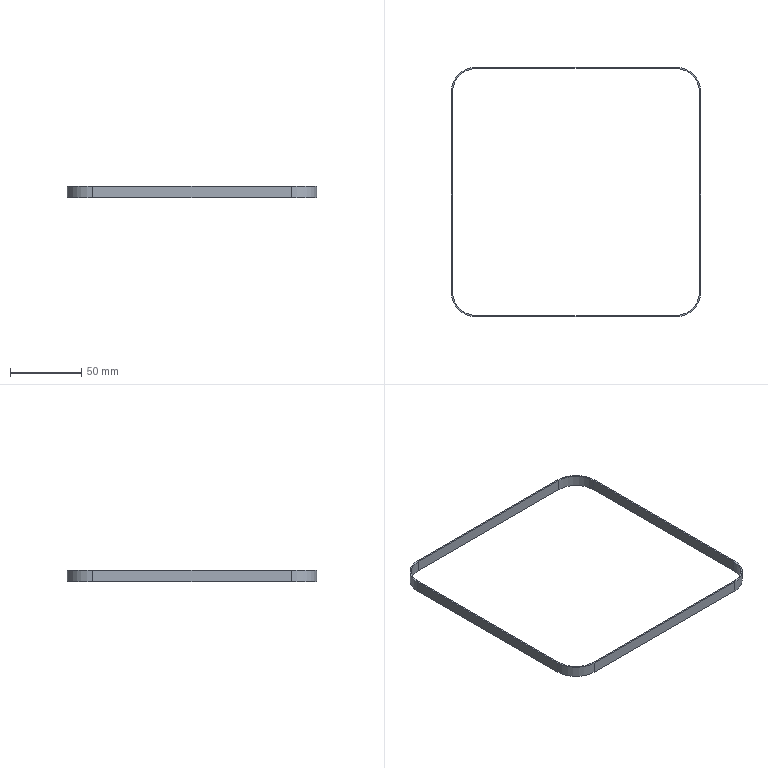Part | NX | features BREP 1 | 1 solid | 18 faces | box 176 x 176 x 7.9 mm | volume 5293 mm3 | plane 10 | cylinder 8 | commonest cylinder face diameters 34 x4 36 x4
STEP:
#1=CARTESIAN_POINT('',(105.422,99.098,7.9));
#2=VERTEX_POINT('',#1);
#3=CARTESIAN_POINT('',(87.422,117.098,7.9));
#4=VERTEX_POINT('',#3);
#5=CARTESIAN_POINT('',(87.422,99.098,7.9));
#6=DIRECTION('',(0.,0.,1.));
#7=DIRECTION('',(1.,0.,0.));
#8=AXIS2_PLACEMENT_3D('',#5,#6,#7);
#9=CIRCLE('',#8,18.);
#10=EDGE_CURVE('',#2,#4,#9,.T.);
#11=ORIENTED_EDGE('',*,*,#10,.T.);
#12=CARTESIAN_POINT('',(-52.578,117.098,7.9));
#13=VERTEX_POINT('',#12);
#14=CARTESIAN_POINT('',(87.422,117.098,7.9));
#15=DIRECTION('',(-1.,0.,0.));
#16=VECTOR('',#15,1000.);
#17=LINE('',#14,#16);
#18=EDGE_CURVE('',#4,#13,#17,.T.);
#19=ORIENTED_EDGE('',*,*,#18,.T.);
#20=CARTESIAN_POINT('',(-70.578,99.098,7.9));
#21=VERTEX_POINT('',#20);
#22=CARTESIAN_POINT('',(-52.578,99.098,7.9));
#23=DIRECTION('',(0.,0.,1.));
#24=DIRECTION('',(1.,0.,0.));
#25=AXIS2_PLACEMENT_3D('',#22,#23,#24);
#26=CIRCLE('',#25,18.);
#27=EDGE_CURVE('',#13,#21,#26,.T.);
#28=ORIENTED_EDGE('',*,*,#27,.T.);
#29=CARTESIAN_POINT('',(-70.578,-40.902,7.9));
#30=VERTEX_POINT('',#29);
#31=CARTESIAN_POINT('',(-70.578,99.098,7.9));
#32=DIRECTION('',(0.,-1.,0.));
#33=VECTOR('',#32,1000.);
#34=LINE('',#31,#33);
#35=EDGE_CURVE('',#21,#30,#34,.T.);
#36=ORIENTED_EDGE('',*,*,#35,.T.);
#37=CARTESIAN_POINT('',(-52.578,-58.902,7.9));
#38=VERTEX_POINT('',#37);
#39=CARTESIAN_POINT('',(-52.578,-40.902,7.9));
#40=DIRECTION('',(0.,0.,1.));
#41=DIRECTION('',(1.,0.,0.));
#42=AXIS2_PLACEMENT_3D('',#39,#40,#41);
#43=CIRCLE('',#42,18.);
#44=EDGE_CURVE('',#30,#38,#43,.T.);
#45=ORIENTED_EDGE('',*,*,#44,.T.);
#46=CARTESIAN_POINT('',(87.422,-58.902,7.9));
#47=VERTEX_POINT('',#46);
#48=CARTESIAN_POINT('',(-52.578,-58.902,7.9));
#49=DIRECTION('',(1.,0.,0.));
#50=VECTOR('',#49,1000.);
#51=LINE('',#48,#50);
#52=EDGE_CURVE('',#38,#47,#51,.T.);
#53=ORIENTED_EDGE('',*,*,#52,.T.);
#54=CARTESIAN_POINT('',(105.422,-40.902,7.9));
#55=VERTEX_POINT('',#54);
#56=CARTESIAN_POINT('',(87.422,-40.902,7.9));
#57=DIRECTION('',(0.,0.,1.));
#58=DIRECTION('',(1.,0.,0.));
#59=AXIS2_PLACEMENT_3D('',#56,#57,#58);
#60=CIRCLE('',#59,18.);
#61=EDGE_CURVE('',#47,#55,#60,.T.);
#62=ORIENTED_EDGE('',*,*,#61,.T.);
#63=CARTESIAN_POINT('',(105.422,-40.902,7.9));
#64=DIRECTION('',(0.,1.,0.));
#65=VECTOR('',#64,1000.);
#66=LINE('',#63,#65);
#67=EDGE_CURVE('',#55,#2,#66,.T.);
#68=ORIENTED_EDGE('',*,*,#67,.T.);
#69=EDGE_LOOP('',(#11,#19,#28,#36,#45,#53,#62,#68));
#70=FACE_BOUND('',#69,.T.);
#71=CARTESIAN_POINT('',(104.422,-40.902,7.9));
#72=VERTEX_POINT('',#71);
#73=CARTESIAN_POINT('',(104.422,99.098,7.9));
#74=VERTEX_POINT('',#73);
#75=CARTESIAN_POINT('',(104.422,-40.902,7.9));
#76=DIRECTION('',(0.,1.,0.));
#77=VECTOR('',#76,1000.);
#78=LINE('',#75,#77);
#79=EDGE_CURVE('',#72,#74,#78,.T.);
#80=ORIENTED_EDGE('',*,*,#79,.F.);
#81=CARTESIAN_POINT('',(87.422,-57.902,7.9));
#82=VERTEX_POINT('',#81);
#83=CARTESIAN_POINT('',(87.422,-40.902,7.9));
#84=DIRECTION('',(0.,0.,1.));
#85=DIRECTION('',(1.,0.,0.));
#86=AXIS2_PLACEMENT_3D('',#83,#84,#85);
#87=CIRCLE('',#86,17.);
#88=EDGE_CURVE('',#82,#72,#87,.T.);
#89=ORIENTED_EDGE('',*,*,#88,.F.);
#90=CARTESIAN_POINT('',(-52.578,-57.902,7.9));
#91=VERTEX_POINT('',#90);
#92=CARTESIAN_POINT('',(-52.578,-57.902,7.9));
#93=DIRECTION('',(1.,0.,0.));
#94=VECTOR('',#93,1000.);
#95=LINE('',#92,#94);
#96=EDGE_CURVE('',#91,#82,#95,.T.);
#97=ORIENTED_EDGE('',*,*,#96,.F.);
#98=CARTESIAN_POINT('',(-69.578,-40.902,7.9));
#99=VERTEX_POINT('',#98);
#100=CARTESIAN_POINT('',(-52.578,-40.902,7.9));
#101=DIRECTION('',(0.,0.,1.));
#102=DIRECTION('',(1.,0.,0.));
#103=AXIS2_PLACEMENT_3D('',#100,#101,#102);
#104=CIRCLE('',#103,17.);
#105=EDGE_CURVE('',#99,#91,#104,.T.);
#106=ORIENTED_EDGE('',*,*,#105,.F.);
#107=CARTESIAN_POINT('',(-69.578,99.098,7.9));
#108=VERTEX_POINT('',#107);
#109=CARTESIAN_POINT('',(-69.578,99.098,7.9));
#110=DIRECTION('',(0.,-1.,0.));
#111=VECTOR('',#110,1000.);
#112=LINE('',#109,#111);
#113=EDGE_CURVE('',#108,#99,#112,.T.);
#114=ORIENTED_EDGE('',*,*,#113,.F.);
#115=CARTESIAN_POINT('',(-52.578,116.098,7.9));
#116=VERTEX_POINT('',#115);
#117=CARTESIAN_POINT('',(-52.578,99.098,7.9));
#118=DIRECTION('',(0.,0.,1.));
#119=DIRECTION('',(1.,0.,0.));
#120=AXIS2_PLACEMENT_3D('',#117,#118,#119);
#121=CIRCLE('',#120,17.);
#122=EDGE_CURVE('',#116,#108,#121,.T.);
#123=ORIENTED_EDGE('',*,*,#122,.F.);
#124=CARTESIAN_POINT('',(87.422,116.098,7.9));
#125=VERTEX_POINT('',#124);
#126=CARTESIAN_POINT('',(87.422,116.098,7.9));
#127=DIRECTION('',(-1.,0.,0.));
#128=VECTOR('',#127,1000.);
#129=LINE('',#126,#128);
#130=EDGE_CURVE('',#125,#116,#129,.T.);
#131=ORIENTED_EDGE('',*,*,#130,.F.);
#132=CARTESIAN_POINT('',(87.422,99.098,7.9));
#133=DIRECTION('',(0.,0.,1.));
#134=DIRECTION('',(1.,0.,0.));
#135=AXIS2_PLACEMENT_3D('',#132,#133,#134);
#136=CIRCLE('',#135,17.);
#137=EDGE_CURVE('',#74,#125,#136,.T.);
#138=ORIENTED_EDGE('',*,*,#137,.F.);
#139=EDGE_LOOP('',(#80,#89,#97,#106,#114,#123,#131,#138));
#140=FACE_BOUND('',#139,.T.);
#141=CARTESIAN_POINT('',(87.422,99.098,7.9));
#142=DIRECTION('',(0.,0.,1.));
#143=DIRECTION('',(-1.,0.,0.));
#144=AXIS2_PLACEMENT_3D('',#141,#142,#143);
#145=PLANE('',#144);
#146=ADVANCED_FACE('',(#70,#140),#145,.T.);
#147=CARTESIAN_POINT('',(105.422,99.098,0.));
#148=VERTEX_POINT('',#147);
#149=CARTESIAN_POINT('',(87.422,117.098,0.));
#150=VERTEX_POINT('',#149);
#151=CARTESIAN_POINT('',(87.422,99.098,0.));
#152=DIRECTION('',(0.,0.,1.));
#153=DIRECTION('',(1.,0.,0.));
#154=AXIS2_PLACEMENT_3D('',#151,#152,#153);
#155=CIRCLE('',#154,18.);
#156=EDGE_CURVE('',#148,#150,#155,.T.);
#157=ORIENTED_EDGE('',*,*,#156,.F.);
#158=CARTESIAN_POINT('',(105.422,-40.902,0.));
#159=VERTEX_POINT('',#158);
#160=CARTESIAN_POINT('',(105.422,-40.902,0.));
#161=DIRECTION('',(0.,1.,0.));
#162=VECTOR('',#161,1000.);
#163=LINE('',#160,#162);
#164=EDGE_CURVE('',#159,#148,#163,.T.);
#165=ORIENTED_EDGE('',*,*,#164,.F.);
#166=CARTESIAN_POINT('',(87.422,-58.902,0.));
#167=VERTEX_POINT('',#166);
#168=CARTESIAN_POINT('',(87.422,-40.902,0.));
#169=DIRECTION('',(0.,0.,1.));
#170=DIRECTION('',(1.,0.,0.));
#171=AXIS2_PLACEMENT_3D('',#168,#169,#170);
#172=CIRCLE('',#171,18.);
#173=EDGE_CURVE('',#167,#159,#172,.T.);
#174=ORIENTED_EDGE('',*,*,#173,.F.);
#175=CARTESIAN_POINT('',(-52.578,-58.902,0.));
#176=VERTEX_POINT('',#175);
#177=CARTESIAN_POINT('',(-52.578,-58.902,0.));
#178=DIRECTION('',(1.,0.,0.));
#179=VECTOR('',#178,1000.);
#180=LINE('',#177,#179);
#181=EDGE_CURVE('',#176,#167,#180,.T.);
#182=ORIENTED_EDGE('',*,*,#181,.F.);
#183=CARTESIAN_POINT('',(-70.578,-40.902,0.));
#184=VERTEX_POINT('',#183);
#185=CARTESIAN_POINT('',(-52.578,-40.902,0.));
#186=DIRECTION('',(0.,0.,1.));
#187=DIRECTION('',(1.,0.,0.));
#188=AXIS2_PLACEMENT_3D('',#185,#186,#187);
#189=CIRCLE('',#188,18.);
#190=EDGE_CURVE('',#184,#176,#189,.T.);
#191=ORIENTED_EDGE('',*,*,#190,.F.);
#192=CARTESIAN_POINT('',(-70.578,99.098,0.));
#193=VERTEX_POINT('',#192);
#194=CARTESIAN_POINT('',(-70.578,99.098,0.));
#195=DIRECTION('',(0.,-1.,0.));
#196=VECTOR('',#195,1000.);
#197=LINE('',#194,#196);
#198=EDGE_CURVE('',#193,#184,#197,.T.);
#199=ORIENTED_EDGE('',*,*,#198,.F.);
#200=CARTESIAN_POINT('',(-52.578,117.098,0.));
#201=VERTEX_POINT('',#200);
#202=CARTESIAN_POINT('',(-52.578,99.098,0.));
#203=DIRECTION('',(0.,0.,1.));
#204=DIRECTION('',(1.,0.,0.));
#205=AXIS2_PLACEMENT_3D('',#202,#203,#204);
#206=CIRCLE('',#205,18.);
#207=EDGE_CURVE('',#201,#193,#206,.T.);
#208=ORIENTED_EDGE('',*,*,#207,.F.);
#209=CARTESIAN_POINT('',(87.422,117.098,0.));
#210=DIRECTION('',(-1.,0.,0.));
#211=VECTOR('',#210,1000.);
#212=LINE('',#209,#211);
#213=EDGE_CURVE('',#150,#201,#212,.T.);
#214=ORIENTED_EDGE('',*,*,#213,.F.);
#215=EDGE_LOOP('',(#157,#165,#174,#182,#191,#199,#208,#214));
#216=FACE_BOUND('',#215,.T.);
#217=CARTESIAN_POINT('',(87.422,-57.902,0.));
#218=VERTEX_POINT('',#217);
#219=CARTESIAN_POINT('',(104.422,-40.902,0.));
#220=VERTEX_POINT('',#219);
#221=CARTESIAN_POINT('',(87.422,-40.902,0.));
#222=DIRECTION('',(0.,0.,1.));
#223=DIRECTION('',(1.,0.,0.));
#224=AXIS2_PLACEMENT_3D('',#221,#222,#223);
#225=CIRCLE('',#224,17.);
#226=EDGE_CURVE('',#218,#220,#225,.T.);
#227=ORIENTED_EDGE('',*,*,#226,.T.);
#228=CARTESIAN_POINT('',(104.422,99.098,0.));
#229=VERTEX_POINT('',#228);
#230=CARTESIAN_POINT('',(104.422,-40.902,0.));
#231=DIRECTION('',(0.,1.,0.));
#232=VECTOR('',#231,1000.);
#233=LINE('',#230,#232);
#234=EDGE_CURVE('',#220,#229,#233,.T.);
#235=ORIENTED_EDGE('',*,*,#234,.T.);
#236=CARTESIAN_POINT('',(87.422,116.098,0.));
#237=VERTEX_POINT('',#236);
#238=CARTESIAN_POINT('',(87.422,99.098,0.));
#239=DIRECTION('',(0.,0.,1.));
#240=DIRECTION('',(1.,0.,0.));
#241=AXIS2_PLACEMENT_3D('',#238,#239,#240);
#242=CIRCLE('',#241,17.);
#243=EDGE_CURVE('',#229,#237,#242,.T.);
#244=ORIENTED_EDGE('',*,*,#243,.T.);
#245=CARTESIAN_POINT('',(-52.578,116.098,0.));
#246=VERTEX_POINT('',#245);
#247=CARTESIAN_POINT('',(87.422,116.098,0.));
#248=DIRECTION('',(-1.,0.,0.));
#249=VECTOR('',#248,1000.);
#250=LINE('',#247,#249);
#251=EDGE_CURVE('',#237,#246,#250,.T.);
#252=ORIENTED_EDGE('',*,*,#251,.T.);
#253=CARTESIAN_POINT('',(-69.578,99.098,0.));
#254=VERTEX_POINT('',#253);
#255=CARTESIAN_POINT('',(-52.578,99.098,0.));
#256=DIRECTION('',(0.,0.,1.));
#257=DIRECTION('',(1.,0.,0.));
#258=AXIS2_PLACEMENT_3D('',#255,#256,#257);
#259=CIRCLE('',#258,17.);
#260=EDGE_CURVE('',#246,#254,#259,.T.);
#261=ORIENTED_EDGE('',*,*,#260,.T.);
#262=CARTESIAN_POINT('',(-69.578,-40.902,0.));
#263=VERTEX_POINT('',#262);
#264=CARTESIAN_POINT('',(-69.578,99.098,0.));
#265=DIRECTION('',(0.,-1.,0.));
#266=VECTOR('',#265,1000.);
#267=LINE('',#264,#266);
#268=EDGE_CURVE('',#254,#263,#267,.T.);
#269=ORIENTED_EDGE('',*,*,#268,.T.);
#270=CARTESIAN_POINT('',(-52.578,-57.902,0.));
#271=VERTEX_POINT('',#270);
#272=CARTESIAN_POINT('',(-52.578,-40.902,0.));
#273=DIRECTION('',(0.,0.,1.));
#274=DIRECTION('',(1.,0.,0.));
#275=AXIS2_PLACEMENT_3D('',#272,#273,#274);
#276=CIRCLE('',#275,17.);
#277=EDGE_CURVE('',#263,#271,#276,.T.);
#278=ORIENTED_EDGE('',*,*,#277,.T.);
#279=CARTESIAN_POINT('',(-52.578,-57.902,0.));
#280=DIRECTION('',(1.,0.,0.));
#281=VECTOR('',#280,1000.);
#282=LINE('',#279,#281);
#283=EDGE_CURVE('',#271,#218,#282,.T.);
#284=ORIENTED_EDGE('',*,*,#283,.T.);
#285=EDGE_LOOP('',(#227,#235,#244,#252,#261,#269,#278,#284));
#286=FACE_BOUND('',#285,.T.);
#287=CARTESIAN_POINT('',(87.422,99.098,0.));
#288=DIRECTION('',(0.,0.,1.));
#289=DIRECTION('',(-1.,0.,0.));
#290=AXIS2_PLACEMENT_3D('',#287,#288,#289);
#291=PLANE('',#290);
#292=ADVANCED_FACE('',(#216,#286),#291,.F.);
#293=ORIENTED_EDGE('',*,*,#156,.T.);
#294=CARTESIAN_POINT('',(87.422,117.098,7.9));
#295=DIRECTION('',(0.,0.,-1.));
#296=VECTOR('',#295,1000.);
#297=LINE('',#294,#296);
#298=EDGE_CURVE('',#4,#150,#297,.T.);
#299=ORIENTED_EDGE('',*,*,#298,.F.);
#300=ORIENTED_EDGE('',*,*,#10,.F.);
#301=CARTESIAN_POINT('',(105.422,99.098,7.9));
#302=DIRECTION('',(0.,0.,-1.));
#303=VECTOR('',#302,1000.);
#304=LINE('',#301,#303);
#305=EDGE_CURVE('',#2,#148,#304,.T.);
#306=ORIENTED_EDGE('',*,*,#305,.T.);
#307=EDGE_LOOP('',(#293,#299,#300,#306));
#308=FACE_BOUND('',#307,.T.);
#309=CARTESIAN_POINT('',(87.422,99.098,7.9));
#310=DIRECTION('',(0.,0.,-1.));
#311=DIRECTION('',(1.,0.,0.));
#312=AXIS2_PLACEMENT_3D('',#309,#310,#311);
#313=CYLINDRICAL_SURFACE('',#312,18.);
#314=ADVANCED_FACE('',(#308),#313,.T.);
#315=ORIENTED_EDGE('',*,*,#213,.T.);
#316=CARTESIAN_POINT('',(-52.578,117.098,7.9));
#317=DIRECTION('',(0.,0.,-1.));
#318=VECTOR('',#317,1000.);
#319=LINE('',#316,#318);
#320=EDGE_CURVE('',#13,#201,#319,.T.);
#321=ORIENTED_EDGE('',*,*,#320,.F.);
#322=ORIENTED_EDGE('',*,*,#18,.F.);
#323=ORIENTED_EDGE('',*,*,#298,.T.);
#324=EDGE_LOOP('',(#315,#321,#322,#323));
#325=FACE_BOUND('',#324,.T.);
#326=CARTESIAN_POINT('',(87.422,117.098,7.9));
#327=DIRECTION('',(0.,-1.,0.));
#328=DIRECTION('',(0.,0.,1.));
#329=AXIS2_PLACEMENT_3D('',#326,#327,#328);
#330=PLANE('',#329);
#331=ADVANCED_FACE('',(#325),#330,.F.);
#332=ORIENTED_EDGE('',*,*,#207,.T.);
#333=CARTESIAN_POINT('',(-70.578,99.098,7.9));
#334=DIRECTION('',(0.,0.,-1.));
#335=VECTOR('',#334,1000.);
#336=LINE('',#333,#335);
#337=EDGE_CURVE('',#21,#193,#336,.T.);
#338=ORIENTED_EDGE('',*,*,#337,.F.);
#339=ORIENTED_EDGE('',*,*,#27,.F.);
#340=ORIENTED_EDGE('',*,*,#320,.T.);
#341=EDGE_LOOP('',(#332,#338,#339,#340));
#342=FACE_BOUND('',#341,.T.);
#343=CARTESIAN_POINT('',(-52.578,99.098,7.9));
#344=DIRECTION('',(0.,0.,-1.));
#345=DIRECTION('',(1.,0.,0.));
#346=AXIS2_PLACEMENT_3D('',#343,#344,#345);
#347=CYLINDRICAL_SURFACE('',#346,18.);
#348=ADVANCED_FACE('',(#342),#347,.T.);
#349=ORIENTED_EDGE('',*,*,#198,.T.);
#350=CARTESIAN_POINT('',(-70.578,-40.902,7.9));
#351=DIRECTION('',(0.,0.,-1.));
#352=VECTOR('',#351,1000.);
#353=LINE('',#350,#352);
#354=EDGE_CURVE('',#30,#184,#353,.T.);
#355=ORIENTED_EDGE('',*,*,#354,.F.);
#356=ORIENTED_EDGE('',*,*,#35,.F.);
#357=ORIENTED_EDGE('',*,*,#337,.T.);
#358=EDGE_LOOP('',(#349,#355,#356,#357));
#359=FACE_BOUND('',#358,.T.);
#360=CARTESIAN_POINT('',(-70.578,99.098,7.9));
#361=DIRECTION('',(1.,0.,0.));
#362=DIRECTION('',(0.,-1.,0.));
#363=AXIS2_PLACEMENT_3D('',#360,#361,#362);
#364=PLANE('',#363);
#365=ADVANCED_FACE('',(#359),#364,.F.);
#366=ORIENTED_EDGE('',*,*,#190,.T.);
#367=CARTESIAN_POINT('',(-52.578,-58.902,7.9));
#368=DIRECTION('',(0.,0.,-1.));
#369=VECTOR('',#368,1000.);
#370=LINE('',#367,#369);
#371=EDGE_CURVE('',#38,#176,#370,.T.);
#372=ORIENTED_EDGE('',*,*,#371,.F.);
#373=ORIENTED_EDGE('',*,*,#44,.F.);
#374=ORIENTED_EDGE('',*,*,#354,.T.);
#375=EDGE_LOOP('',(#366,#372,#373,#374));
#376=FACE_BOUND('',#375,.T.);
#377=CARTESIAN_POINT('',(-52.578,-40.902,7.9));
#378=DIRECTION('',(0.,0.,-1.));
#379=DIRECTION('',(1.,0.,0.));
#380=AXIS2_PLACEMENT_3D('',#377,#378,#379);
#381=CYLINDRICAL_SURFACE('',#380,18.);
#382=ADVANCED_FACE('',(#376),#381,.T.);
#383=ORIENTED_EDGE('',*,*,#181,.T.);
#384=CARTESIAN_POINT('',(87.422,-58.902,7.9));
#385=DIRECTION('',(0.,0.,-1.));
#386=VECTOR('',#385,1000.);
#387=LINE('',#384,#386);
#388=EDGE_CURVE('',#47,#167,#387,.T.);
#389=ORIENTED_EDGE('',*,*,#388,.F.);
#390=ORIENTED_EDGE('',*,*,#52,.F.);
#391=ORIENTED_EDGE('',*,*,#371,.T.);
#392=EDGE_LOOP('',(#383,#389,#390,#391));
#393=FACE_BOUND('',#392,.T.);
#394=CARTESIAN_POINT('',(-52.578,-58.902,7.9));
#395=DIRECTION('',(0.,1.,0.));
#396=DIRECTION('',(-1.,0.,0.));
#397=AXIS2_PLACEMENT_3D('',#394,#395,#396);
#398=PLANE('',#397);
#399=ADVANCED_FACE('',(#393),#398,.F.);
#400=ORIENTED_EDGE('',*,*,#173,.T.);
#401=CARTESIAN_POINT('',(105.422,-40.902,7.9));
#402=DIRECTION('',(0.,0.,-1.));
#403=VECTOR('',#402,1000.);
#404=LINE('',#401,#403);
#405=EDGE_CURVE('',#55,#159,#404,.T.);
#406=ORIENTED_EDGE('',*,*,#405,.F.);
#407=ORIENTED_EDGE('',*,*,#61,.F.);
#408=ORIENTED_EDGE('',*,*,#388,.T.);
#409=EDGE_LOOP('',(#400,#406,#407,#408));
#410=FACE_BOUND('',#409,.T.);
#411=CARTESIAN_POINT('',(87.422,-40.902,7.9));
#412=DIRECTION('',(0.,0.,-1.));
#413=DIRECTION('',(1.,0.,0.));
#414=AXIS2_PLACEMENT_3D('',#411,#412,#413);
#415=CYLINDRICAL_SURFACE('',#414,18.);
#416=ADVANCED_FACE('',(#410),#415,.T.);
#417=ORIENTED_EDGE('',*,*,#164,.T.);
#418=ORIENTED_EDGE('',*,*,#305,.F.);
#419=ORIENTED_EDGE('',*,*,#67,.F.);
#420=ORIENTED_EDGE('',*,*,#405,.T.);
#421=EDGE_LOOP('',(#417,#418,#419,#420));
#422=FACE_BOUND('',#421,.T.);
#423=CARTESIAN_POINT('',(105.422,-40.902,7.9));
#424=DIRECTION('',(-1.,0.,0.));
#425=DIRECTION('',(0.,0.,-1.));
#426=AXIS2_PLACEMENT_3D('',#423,#424,#425);
#427=PLANE('',#426);
#428=ADVANCED_FACE('',(#422),#427,.F.);
#429=ORIENTED_EDGE('',*,*,#226,.F.);
#430=CARTESIAN_POINT('',(87.422,-57.902,7.9));
#431=DIRECTION('',(0.,0.,-1.));
#432=VECTOR('',#431,1000.);
#433=LINE('',#430,#432);
#434=EDGE_CURVE('',#82,#218,#433,.T.);
#435=ORIENTED_EDGE('',*,*,#434,.F.);
#436=ORIENTED_EDGE('',*,*,#88,.T.);
#437=CARTESIAN_POINT('',(104.422,-40.902,7.9));
#438=DIRECTION('',(0.,0.,-1.));
#439=VECTOR('',#438,1000.);
#440=LINE('',#437,#439);
#441=EDGE_CURVE('',#72,#220,#440,.T.);
#442=ORIENTED_EDGE('',*,*,#441,.T.);
#443=EDGE_LOOP('',(#429,#435,#436,#442));
#444=FACE_BOUND('',#443,.T.);
#445=CARTESIAN_POINT('',(87.422,-40.902,7.9));
#446=DIRECTION('',(0.,0.,-1.));
#447=DIRECTION('',(1.,0.,0.));
#448=AXIS2_PLACEMENT_3D('',#445,#446,#447);
#449=CYLINDRICAL_SURFACE('',#448,17.);
#450=ADVANCED_FACE('',(#444),#449,.F.);
#451=ORIENTED_EDGE('',*,*,#234,.F.);
#452=ORIENTED_EDGE('',*,*,#441,.F.);
#453=ORIENTED_EDGE('',*,*,#79,.T.);
#454=CARTESIAN_POINT('',(104.422,99.098,7.9));
#455=DIRECTION('',(0.,0.,-1.));
#456=VECTOR('',#455,1000.);
#457=LINE('',#454,#456);
#458=EDGE_CURVE('',#74,#229,#457,.T.);
#459=ORIENTED_EDGE('',*,*,#458,.T.);
#460=EDGE_LOOP('',(#451,#452,#453,#459));
#461=FACE_BOUND('',#460,.T.);
#462=CARTESIAN_POINT('',(104.422,-40.902,7.9));
#463=DIRECTION('',(-1.,0.,0.));
#464=DIRECTION('',(0.,0.,-1.));
#465=AXIS2_PLACEMENT_3D('',#462,#463,#464);
#466=PLANE('',#465);
#467=ADVANCED_FACE('',(#461),#466,.T.);
#468=ORIENTED_EDGE('',*,*,#243,.F.);
#469=ORIENTED_EDGE('',*,*,#458,.F.);
#470=ORIENTED_EDGE('',*,*,#137,.T.);
#471=CARTESIAN_POINT('',(87.422,116.098,7.9));
#472=DIRECTION('',(0.,0.,-1.));
#473=VECTOR('',#472,1000.);
#474=LINE('',#471,#473);
#475=EDGE_CURVE('',#125,#237,#474,.T.);
#476=ORIENTED_EDGE('',*,*,#475,.T.);
#477=EDGE_LOOP('',(#468,#469,#470,#476));
#478=FACE_BOUND('',#477,.T.);
#479=CARTESIAN_POINT('',(87.422,99.098,7.9));
#480=DIRECTION('',(0.,0.,-1.));
#481=DIRECTION('',(1.,0.,0.));
#482=AXIS2_PLACEMENT_3D('',#479,#480,#481);
#483=CYLINDRICAL_SURFACE('',#482,17.);
#484=ADVANCED_FACE('',(#478),#483,.F.);
#485=ORIENTED_EDGE('',*,*,#251,.F.);
#486=ORIENTED_EDGE('',*,*,#475,.F.);
#487=ORIENTED_EDGE('',*,*,#130,.T.);
#488=CARTESIAN_POINT('',(-52.578,116.098,7.9));
#489=DIRECTION('',(0.,0.,-1.));
#490=VECTOR('',#489,1000.);
#491=LINE('',#488,#490);
#492=EDGE_CURVE('',#116,#246,#491,.T.);
#493=ORIENTED_EDGE('',*,*,#492,.T.);
#494=EDGE_LOOP('',(#485,#486,#487,#493));
#495=FACE_BOUND('',#494,.T.);
#496=CARTESIAN_POINT('',(87.422,116.098,7.9));
#497=DIRECTION('',(0.,-1.,0.));
#498=DIRECTION('',(0.,0.,1.));
#499=AXIS2_PLACEMENT_3D('',#496,#497,#498);
#500=PLANE('',#499);
#501=ADVANCED_FACE('',(#495),#500,.T.);
#502=ORIENTED_EDGE('',*,*,#260,.F.);
#503=ORIENTED_EDGE('',*,*,#492,.F.);
#504=ORIENTED_EDGE('',*,*,#122,.T.);
#505=CARTESIAN_POINT('',(-69.578,99.098,7.9));
#506=DIRECTION('',(0.,0.,-1.));
#507=VECTOR('',#506,1000.);
#508=LINE('',#505,#507);
#509=EDGE_CURVE('',#108,#254,#508,.T.);
#510=ORIENTED_EDGE('',*,*,#509,.T.);
#511=EDGE_LOOP('',(#502,#503,#504,#510));
#512=FACE_BOUND('',#511,.T.);
#513=CARTESIAN_POINT('',(-52.578,99.098,7.9));
#514=DIRECTION('',(0.,0.,-1.));
#515=DIRECTION('',(1.,0.,0.));
#516=AXIS2_PLACEMENT_3D('',#513,#514,#515);
#517=CYLINDRICAL_SURFACE('',#516,17.);
#518=ADVANCED_FACE('',(#512),#517,.F.);
#519=ORIENTED_EDGE('',*,*,#268,.F.);
#520=ORIENTED_EDGE('',*,*,#509,.F.);
#521=ORIENTED_EDGE('',*,*,#113,.T.);
#522=CARTESIAN_POINT('',(-69.578,-40.902,7.9));
#523=DIRECTION('',(0.,0.,-1.));
#524=VECTOR('',#523,1000.);
#525=LINE('',#522,#524);
#526=EDGE_CURVE('',#99,#263,#525,.T.);
#527=ORIENTED_EDGE('',*,*,#526,.T.);
#528=EDGE_LOOP('',(#519,#520,#521,#527));
#529=FACE_BOUND('',#528,.T.);
#530=CARTESIAN_POINT('',(-69.578,99.098,7.9));
#531=DIRECTION('',(1.,0.,0.));
#532=DIRECTION('',(0.,-1.,0.));
#533=AXIS2_PLACEMENT_3D('',#530,#531,#532);
#534=PLANE('',#533);
#535=ADVANCED_FACE('',(#529),#534,.T.);
#536=ORIENTED_EDGE('',*,*,#277,.F.);
#537=ORIENTED_EDGE('',*,*,#526,.F.);
#538=ORIENTED_EDGE('',*,*,#105,.T.);
#539=CARTESIAN_POINT('',(-52.578,-57.902,7.9));
#540=DIRECTION('',(0.,0.,-1.));
#541=VECTOR('',#540,1000.);
#542=LINE('',#539,#541);
#543=EDGE_CURVE('',#91,#271,#542,.T.);
#544=ORIENTED_EDGE('',*,*,#543,.T.);
#545=EDGE_LOOP('',(#536,#537,#538,#544));
#546=FACE_BOUND('',#545,.T.);
#547=CARTESIAN_POINT('',(-52.578,-40.902,7.9));
#548=DIRECTION('',(0.,0.,-1.));
#549=DIRECTION('',(1.,0.,0.));
#550=AXIS2_PLACEMENT_3D('',#547,#548,#549);
#551=CYLINDRICAL_SURFACE('',#550,17.);
#552=ADVANCED_FACE('',(#546),#551,.F.);
#553=ORIENTED_EDGE('',*,*,#283,.F.);
#554=ORIENTED_EDGE('',*,*,#543,.F.);
#555=ORIENTED_EDGE('',*,*,#96,.T.);
#556=ORIENTED_EDGE('',*,*,#434,.T.);
#557=EDGE_LOOP('',(#553,#554,#555,#556));
#558=FACE_BOUND('',#557,.T.);
#559=CARTESIAN_POINT('',(-52.578,-57.902,7.9));
#560=DIRECTION('',(0.,1.,0.));
#561=DIRECTION('',(-1.,0.,0.));
#562=AXIS2_PLACEMENT_3D('',#559,#560,#561);
#563=PLANE('',#562);
#564=ADVANCED_FACE('',(#558),#563,.T.);
#565=CLOSED_SHELL('',(#146,#292,#314,#331,#348,#365,#382,#399,#416,#428,#450,#467,#484,#501,#518,#535,#552,#564));
#566=MANIFOLD_SOLID_BREP('',#565);
#567=(LENGTH_UNIT()NAMED_UNIT(*)SI_UNIT(.MILLI.,.METRE.));
#568=UNCERTAINTY_MEASURE_WITH_UNIT(LENGTH_MEASURE(0.00001),#567,'','');
#569=(NAMED_UNIT(*)PLANE_ANGLE_UNIT()SI_UNIT($,.RADIAN.));
#570=(NAMED_UNIT(*)SI_UNIT($,.STERADIAN.)SOLID_ANGLE_UNIT());
#571=(GEOMETRIC_REPRESENTATION_CONTEXT(3)GLOBAL_UNCERTAINTY_ASSIGNED_CONTEXT((#568))GLOBAL_UNIT_ASSIGNED_CONTEXT((#567,#569,#570))REPRESENTATION_CONTEXT('',''));
#572=ADVANCED_BREP_SHAPE_REPRESENTATION('',(#566),#571);